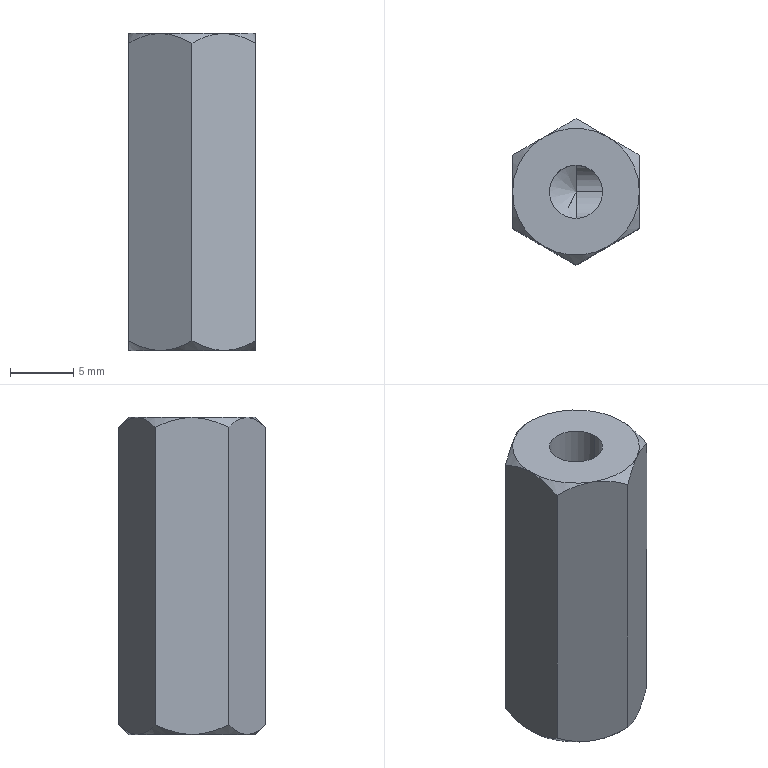Part | SolidWorks | features HoleWzd 3, RevCut 2, Extrusion 1, ICE 1 | 1 solid | 30 faces | box 10 x 11.547 x 25 mm | volume 1883 mm3 | cone 15 | plane 9 | cylinder 6 | commonest cylinder face diameters 4.2 x4 3.3 x2
STEP:
#1=CARTESIAN_POINT('',(1.65,0.,9.));
#2=VERTEX_POINT('',#1);
#3=CARTESIAN_POINT('',(-1.65,0.,9.));
#4=VERTEX_POINT('',#3);
#5=CARTESIAN_POINT('',(0.,0.,9.));
#6=DIRECTION('',(0.,0.,-1.));
#7=DIRECTION('',(-1.,0.,0.));
#8=AXIS2_PLACEMENT_3D('',#5,#6,#7);
#9=CIRCLE('',#8,1.65);
#10=EDGE_CURVE('',#2,#4,#9,.T.);
#11=ORIENTED_EDGE('',*,*,#10,.F.);
#12=CARTESIAN_POINT('',(1.65,0.,0.));
#13=VERTEX_POINT('',#12);
#14=CARTESIAN_POINT('',(1.65,0.,0.));
#15=DIRECTION('',(0.,0.,-1.));
#16=VECTOR('',#15,1000.);
#17=LINE('',#14,#16);
#18=EDGE_CURVE('',#2,#13,#17,.T.);
#19=ORIENTED_EDGE('',*,*,#18,.T.);
#20=CARTESIAN_POINT('',(-1.65,0.,0.));
#21=VERTEX_POINT('',#20);
#22=CARTESIAN_POINT('',(0.,0.,0.));
#23=DIRECTION('',(0.,0.,-1.));
#24=DIRECTION('',(-1.,0.,0.));
#25=AXIS2_PLACEMENT_3D('',#22,#23,#24);
#26=CIRCLE('',#25,1.65);
#27=EDGE_CURVE('',#13,#21,#26,.T.);
#28=ORIENTED_EDGE('',*,*,#27,.T.);
#29=CARTESIAN_POINT('',(-1.65,0.,0.));
#30=DIRECTION('',(0.,0.,-1.));
#31=VECTOR('',#30,1000.);
#32=LINE('',#29,#31);
#33=EDGE_CURVE('',#4,#21,#32,.T.);
#34=ORIENTED_EDGE('',*,*,#33,.F.);
#35=EDGE_LOOP('',(#11,#19,#28,#34));
#36=FACE_OUTER_BOUND('',#35,.T.);
#37=CARTESIAN_POINT('',(0.,0.,0.));
#38=DIRECTION('',(0.,0.,-1.));
#39=DIRECTION('',(-1.,0.,0.));
#40=AXIS2_PLACEMENT_3D('',#37,#38,#39);
#41=CYLINDRICAL_SURFACE('',#40,1.65);
#42=ADVANCED_FACE('',(#36),#41,.F.);
#43=CARTESIAN_POINT('',(0.,0.,9.991));
#44=VERTEX_POINT('',#43);
#45=CARTESIAN_POINT('',(-1.65,0.,9.));
#46=DIRECTION('',(-0.8572,0.,-0.515));
#47=VECTOR('',#46,1000.);
#48=LINE('',#45,#47);
#49=EDGE_CURVE('',#44,#4,#48,.T.);
#50=ORIENTED_EDGE('',*,*,#49,.F.);
#51=CARTESIAN_POINT('',(1.65,0.,9.));
#52=DIRECTION('',(0.8572,0.,-0.515));
#53=VECTOR('',#52,1000.);
#54=LINE('',#51,#53);
#55=EDGE_CURVE('',#44,#2,#54,.T.);
#56=ORIENTED_EDGE('',*,*,#55,.T.);
#57=ORIENTED_EDGE('',*,*,#10,.T.);
#58=EDGE_LOOP('',(#50,#56,#57));
#59=FACE_OUTER_BOUND('',#58,.T.);
#60=CARTESIAN_POINT('',(0.,0.,9.));
#61=DIRECTION('',(0.,0.,-1.));
#62=DIRECTION('',(-1.,0.,0.));
#63=AXIS2_PLACEMENT_3D('',#60,#61,#62);
#64=CONICAL_SURFACE('',#63,1.65,1.03);
#65=ADVANCED_FACE('',(#59),#64,.F.);
#66=CARTESIAN_POINT('',(5.,0.,12.9));
#67=VERTEX_POINT('',#66);
#68=CARTESIAN_POINT('',(5.,0.,17.1));
#69=VERTEX_POINT('',#68);
#70=CARTESIAN_POINT('',(5.,0.,15.));
#71=DIRECTION('',(-1.,0.,0.));
#72=DIRECTION('',(0.,0.,1.));
#73=AXIS2_PLACEMENT_3D('',#70,#71,#72);
#74=CIRCLE('',#73,2.1);
#75=EDGE_CURVE('',#67,#69,#74,.T.);
#76=ORIENTED_EDGE('',*,*,#75,.F.);
#77=CARTESIAN_POINT('',(0.,0.,12.9));
#78=VERTEX_POINT('',#77);
#79=CARTESIAN_POINT('',(0.,0.,12.9));
#80=DIRECTION('',(-1.,0.,0.));
#81=VECTOR('',#80,1000.);
#82=LINE('',#79,#81);
#83=EDGE_CURVE('',#67,#78,#82,.T.);
#84=ORIENTED_EDGE('',*,*,#83,.T.);
#85=CARTESIAN_POINT('',(0.,-2.1,15.));
#86=VERTEX_POINT('',#85);
#87=CARTESIAN_POINT('',(0.,0.,15.));
#88=DIRECTION('',(-1.,0.,0.));
#89=DIRECTION('',(0.,0.,1.));
#90=AXIS2_PLACEMENT_3D('',#87,#88,#89);
#91=CIRCLE('',#90,2.1);
#92=EDGE_CURVE('',#78,#86,#91,.T.);
#93=ORIENTED_EDGE('',*,*,#92,.T.);
#94=CARTESIAN_POINT('',(2.1,0.,17.1));
#95=VERTEX_POINT('',#94);
#96=CARTESIAN_POINT('',(2.1,0.,17.1));
#97=CARTESIAN_POINT('',(2.1,-1.23,17.1));
#98=CARTESIAN_POINT('',(1.23,-2.1,16.23));
#99=CARTESIAN_POINT('',(0.,-2.1,15.));
#100=(BOUNDED_CURVE()B_SPLINE_CURVE(3,(#96,#97,#98,#99),.UNSPECIFIED.,.F.,.T.)B_SPLINE_CURVE_WITH_KNOTS((4,4),(0.,1.571),.UNSPECIFIED.)CURVE()GEOMETRIC_REPRESENTATION_ITEM()RATIONAL_B_SPLINE_CURVE((1.,0.8047,0.8047,1.))REPRESENTATION_ITEM(''));
#101=EDGE_CURVE('',#95,#86,#100,.T.);
#102=ORIENTED_EDGE('',*,*,#101,.F.);
#103=CARTESIAN_POINT('',(0.,0.,17.1));
#104=DIRECTION('',(-1.,0.,0.));
#105=VECTOR('',#104,1000.);
#106=LINE('',#103,#105);
#107=EDGE_CURVE('',#69,#95,#106,.T.);
#108=ORIENTED_EDGE('',*,*,#107,.F.);
#109=EDGE_LOOP('',(#76,#84,#93,#102,#108));
#110=FACE_OUTER_BOUND('',#109,.T.);
#111=CARTESIAN_POINT('',(0.,0.,15.));
#112=DIRECTION('',(-1.,0.,0.));
#113=DIRECTION('',(0.,0.,1.));
#114=AXIS2_PLACEMENT_3D('',#111,#112,#113);
#115=CYLINDRICAL_SURFACE('',#114,2.1);
#116=ADVANCED_FACE('',(#110),#115,.F.);
#117=CARTESIAN_POINT('',(-2.1,0.,15.));
#118=VERTEX_POINT('',#117);
#119=CARTESIAN_POINT('',(0.,0.,15.));
#120=DIRECTION('',(0.,0.,1.));
#121=DIRECTION('',(1.,0.,0.));
#122=AXIS2_PLACEMENT_3D('',#119,#120,#121);
#123=CIRCLE('',#122,2.1);
#124=EDGE_CURVE('',#118,#86,#123,.T.);
#125=ORIENTED_EDGE('',*,*,#124,.F.);
#126=CARTESIAN_POINT('',(-2.1,0.,25.));
#127=VERTEX_POINT('',#126);
#128=CARTESIAN_POINT('',(-2.1,0.,25.));
#129=DIRECTION('',(0.,0.,1.));
#130=VECTOR('',#129,1000.);
#131=LINE('',#128,#130);
#132=EDGE_CURVE('',#118,#127,#131,.T.);
#133=ORIENTED_EDGE('',*,*,#132,.T.);
#134=CARTESIAN_POINT('',(2.1,0.,25.));
#135=VERTEX_POINT('',#134);
#136=CARTESIAN_POINT('',(0.,0.,25.));
#137=DIRECTION('',(0.,0.,1.));
#138=DIRECTION('',(1.,0.,0.));
#139=AXIS2_PLACEMENT_3D('',#136,#137,#138);
#140=CIRCLE('',#139,2.1);
#141=EDGE_CURVE('',#127,#135,#140,.T.);
#142=ORIENTED_EDGE('',*,*,#141,.T.);
#143=CARTESIAN_POINT('',(2.1,0.,25.));
#144=DIRECTION('',(0.,0.,1.));
#145=VECTOR('',#144,1000.);
#146=LINE('',#143,#145);
#147=EDGE_CURVE('',#95,#135,#146,.T.);
#148=ORIENTED_EDGE('',*,*,#147,.F.);
#149=ORIENTED_EDGE('',*,*,#101,.T.);
#150=EDGE_LOOP('',(#125,#133,#142,#148,#149));
#151=FACE_OUTER_BOUND('',#150,.T.);
#152=CARTESIAN_POINT('',(0.,0.,25.));
#153=DIRECTION('',(0.,0.,1.));
#154=DIRECTION('',(1.,0.,0.));
#155=AXIS2_PLACEMENT_3D('',#152,#153,#154);
#156=CYLINDRICAL_SURFACE('',#155,2.1);
#157=ADVANCED_FACE('',(#151),#156,.F.);
#158=CARTESIAN_POINT('',(5.,2.887,24.226));
#159=VERTEX_POINT('',#158);
#160=CARTESIAN_POINT('',(2.5,4.33,25.));
#161=VERTEX_POINT('',#160);
#162=CARTESIAN_POINT('',(5.,2.887,24.226));
#163=CARTESIAN_POINT('',(4.608,3.113,24.453));
#164=CARTESIAN_POINT('',(4.207,3.345,24.645));
#165=CARTESIAN_POINT('',(3.584,3.704,24.851));
#166=CARTESIAN_POINT('',(3.373,3.826,24.905));
#167=CARTESIAN_POINT('',(2.941,4.075,24.98));
#168=CARTESIAN_POINT('',(2.719,4.204,25.));
#169=CARTESIAN_POINT('',(2.5,4.33,25.));
#170=B_SPLINE_CURVE_WITH_KNOTS('',3,(#162,#163,#164,#165,#166,#167,#168,#169),.UNSPECIFIED.,.F.,.F.,(4,2,2,4),(0.000000254,0.001496,0.002245,0.002993),.UNSPECIFIED.);
#171=EDGE_CURVE('',#159,#161,#170,.T.);
#172=ORIENTED_EDGE('',*,*,#171,.F.);
#173=CARTESIAN_POINT('',(5.,2.887,0.7735));
#174=VERTEX_POINT('',#173);
#175=CARTESIAN_POINT('',(5.,2.887,25.));
#176=DIRECTION('',(0.,0.,-1.));
#177=VECTOR('',#176,1000.);
#178=LINE('',#175,#177);
#179=EDGE_CURVE('',#159,#174,#178,.T.);
#180=ORIENTED_EDGE('',*,*,#179,.T.);
#181=CARTESIAN_POINT('',(2.5,4.33,0.));
#182=VERTEX_POINT('',#181);
#183=CARTESIAN_POINT('',(2.5,4.33,0.));
#184=CARTESIAN_POINT('',(2.935,4.079,0.));
#185=CARTESIAN_POINT('',(3.362,3.832,0.07678));
#186=CARTESIAN_POINT('',(4.205,3.346,0.3535));
#187=CARTESIAN_POINT('',(4.608,3.113,0.5474));
#188=CARTESIAN_POINT('',(5.,2.887,0.7735));
#189=B_SPLINE_CURVE_WITH_KNOTS('',3,(#183,#184,#185,#186,#187,#188),.UNSPECIFIED.,.F.,.F.,(4,2,4),(0.002993,0.004478,0.005964),.UNSPECIFIED.);
#190=EDGE_CURVE('',#182,#174,#189,.T.);
#191=ORIENTED_EDGE('',*,*,#190,.F.);
#192=CARTESIAN_POINT('',(0.,5.774,0.7735));
#193=VERTEX_POINT('',#192);
#194=CARTESIAN_POINT('',(0.,5.774,0.7735));
#195=CARTESIAN_POINT('',(0.392,5.547,0.5472));
#196=CARTESIAN_POINT('',(0.7929,5.316,0.3548));
#197=CARTESIAN_POINT('',(1.416,4.956,0.1492));
#198=CARTESIAN_POINT('',(1.627,4.834,0.0946));
#199=CARTESIAN_POINT('',(2.059,4.585,0.01985));
#200=CARTESIAN_POINT('',(2.281,4.457,0.));
#201=CARTESIAN_POINT('',(2.5,4.33,0.));
#202=B_SPLINE_CURVE_WITH_KNOTS('',3,(#194,#195,#196,#197,#198,#199,#200,#201),.UNSPECIFIED.,.F.,.F.,(4,2,2,4),(0.000000254,0.001496,0.002245,0.002993),.UNSPECIFIED.);
#203=EDGE_CURVE('',#193,#182,#202,.T.);
#204=ORIENTED_EDGE('',*,*,#203,.F.);
#205=CARTESIAN_POINT('',(0.,5.774,24.226));
#206=VERTEX_POINT('',#205);
#207=CARTESIAN_POINT('',(0.,5.774,25.));
#208=DIRECTION('',(0.,0.,-1.));
#209=VECTOR('',#208,1000.);
#210=LINE('',#207,#209);
#211=EDGE_CURVE('',#206,#193,#210,.T.);
#212=ORIENTED_EDGE('',*,*,#211,.F.);
#213=CARTESIAN_POINT('',(2.5,4.33,25.));
#214=CARTESIAN_POINT('',(2.065,4.581,25.));
#215=CARTESIAN_POINT('',(1.638,4.828,24.923));
#216=CARTESIAN_POINT('',(0.7946,5.315,24.647));
#217=CARTESIAN_POINT('',(0.3916,5.547,24.453));
#218=CARTESIAN_POINT('',(0.,5.774,24.226));
#219=B_SPLINE_CURVE_WITH_KNOTS('',3,(#213,#214,#215,#216,#217,#218),.UNSPECIFIED.,.F.,.F.,(4,2,4),(0.002993,0.004478,0.005964),.UNSPECIFIED.);
#220=EDGE_CURVE('',#161,#206,#219,.T.);
#221=ORIENTED_EDGE('',*,*,#220,.F.);
#222=EDGE_LOOP('',(#172,#180,#191,#204,#212,#221));
#223=FACE_OUTER_BOUND('',#222,.T.);
#224=CARTESIAN_POINT('',(5.,2.887,25.));
#225=DIRECTION('',(-0.5,-0.866,0.));
#226=DIRECTION('',(0.866,-0.5,0.));
#227=AXIS2_PLACEMENT_3D('',#224,#225,#226);
#228=PLANE('',#227);
#229=ADVANCED_FACE('',(#223),#228,.F.);
#230=CARTESIAN_POINT('',(-2.5,4.33,25.));
#231=VERTEX_POINT('',#230);
#232=CARTESIAN_POINT('',(0.,5.774,24.226));
#233=CARTESIAN_POINT('',(-0.392,5.547,24.453));
#234=CARTESIAN_POINT('',(-0.7929,5.316,24.645));
#235=CARTESIAN_POINT('',(-1.416,4.956,24.851));
#236=CARTESIAN_POINT('',(-1.627,4.834,24.905));
#237=CARTESIAN_POINT('',(-2.059,4.585,24.98));
#238=CARTESIAN_POINT('',(-2.281,4.457,25.));
#239=CARTESIAN_POINT('',(-2.5,4.33,25.));
#240=B_SPLINE_CURVE_WITH_KNOTS('',3,(#232,#233,#234,#235,#236,#237,#238,#239),.UNSPECIFIED.,.F.,.F.,(4,2,2,4),(0.000000254,0.001496,0.002245,0.002993),.UNSPECIFIED.);
#241=EDGE_CURVE('',#206,#231,#240,.T.);
#242=ORIENTED_EDGE('',*,*,#241,.F.);
#243=ORIENTED_EDGE('',*,*,#211,.T.);
#244=CARTESIAN_POINT('',(-2.5,4.33,0.));
#245=VERTEX_POINT('',#244);
#246=CARTESIAN_POINT('',(-2.5,4.33,0.));
#247=CARTESIAN_POINT('',(-2.065,4.581,0.));
#248=CARTESIAN_POINT('',(-1.638,4.828,0.07678));
#249=CARTESIAN_POINT('',(-0.7946,5.315,0.3535));
#250=CARTESIAN_POINT('',(-0.3916,5.547,0.5474));
#251=CARTESIAN_POINT('',(0.,5.774,0.7735));
#252=B_SPLINE_CURVE_WITH_KNOTS('',3,(#246,#247,#248,#249,#250,#251),.UNSPECIFIED.,.F.,.F.,(4,2,4),(0.002993,0.004478,0.005964),.UNSPECIFIED.);
#253=EDGE_CURVE('',#245,#193,#252,.T.);
#254=ORIENTED_EDGE('',*,*,#253,.F.);
#255=CARTESIAN_POINT('',(-5.,2.887,0.7735));
#256=VERTEX_POINT('',#255);
#257=CARTESIAN_POINT('',(-5.,2.887,0.7735));
#258=CARTESIAN_POINT('',(-4.608,3.113,0.5472));
#259=CARTESIAN_POINT('',(-4.207,3.345,0.3548));
#260=CARTESIAN_POINT('',(-3.584,3.704,0.1492));
#261=CARTESIAN_POINT('',(-3.373,3.826,0.0946));
#262=CARTESIAN_POINT('',(-2.941,4.075,0.01985));
#263=CARTESIAN_POINT('',(-2.719,4.204,0.));
#264=CARTESIAN_POINT('',(-2.5,4.33,0.));
#265=B_SPLINE_CURVE_WITH_KNOTS('',3,(#257,#258,#259,#260,#261,#262,#263,#264),.UNSPECIFIED.,.F.,.F.,(4,2,2,4),(0.000000254,0.001496,0.002245,0.002993),.UNSPECIFIED.);
#266=EDGE_CURVE('',#256,#245,#265,.T.);
#267=ORIENTED_EDGE('',*,*,#266,.F.);
#268=CARTESIAN_POINT('',(-5.,2.887,24.226));
#269=VERTEX_POINT('',#268);
#270=CARTESIAN_POINT('',(-5.,2.887,25.));
#271=DIRECTION('',(0.,0.,-1.));
#272=VECTOR('',#271,1000.);
#273=LINE('',#270,#272);
#274=EDGE_CURVE('',#269,#256,#273,.T.);
#275=ORIENTED_EDGE('',*,*,#274,.F.);
#276=CARTESIAN_POINT('',(-2.5,4.33,25.));
#277=CARTESIAN_POINT('',(-2.935,4.079,25.));
#278=CARTESIAN_POINT('',(-3.362,3.832,24.923));
#279=CARTESIAN_POINT('',(-4.205,3.346,24.647));
#280=CARTESIAN_POINT('',(-4.608,3.113,24.453));
#281=CARTESIAN_POINT('',(-5.,2.887,24.226));
#282=B_SPLINE_CURVE_WITH_KNOTS('',3,(#276,#277,#278,#279,#280,#281),.UNSPECIFIED.,.F.,.F.,(4,2,4),(0.002993,0.004478,0.005964),.UNSPECIFIED.);
#283=EDGE_CURVE('',#231,#269,#282,.T.);
#284=ORIENTED_EDGE('',*,*,#283,.F.);
#285=EDGE_LOOP('',(#242,#243,#254,#267,#275,#284));
#286=FACE_OUTER_BOUND('',#285,.T.);
#287=CARTESIAN_POINT('',(0.,5.774,25.));
#288=DIRECTION('',(0.5,-0.866,0.));
#289=DIRECTION('',(0.866,0.5,0.));
#290=AXIS2_PLACEMENT_3D('',#287,#288,#289);
#291=PLANE('',#290);
#292=ADVANCED_FACE('',(#286),#291,.F.);
#293=CARTESIAN_POINT('',(-5.,0.,25.));
#294=VERTEX_POINT('',#293);
#295=CARTESIAN_POINT('',(-5.,2.887,24.226));
#296=CARTESIAN_POINT('',(-5.,2.663,24.338));
#297=CARTESIAN_POINT('',(-5.,2.435,24.443));
#298=CARTESIAN_POINT('',(-5.,1.967,24.631));
#299=CARTESIAN_POINT('',(-5.,1.726,24.715));
#300=CARTESIAN_POINT('',(-5.,1.001,24.922));
#301=CARTESIAN_POINT('',(-5.,0.5067,25.));
#302=CARTESIAN_POINT('',(-5.,0.,25.));
#303=B_SPLINE_CURVE_WITH_KNOTS('',3,(#295,#296,#297,#298,#299,#300,#301,#302),.UNSPECIFIED.,.F.,.F.,(4,2,2,4),(0.007249,0.008002,0.008755,0.01026),.UNSPECIFIED.);
#304=EDGE_CURVE('',#269,#294,#303,.T.);
#305=ORIENTED_EDGE('',*,*,#304,.F.);
#306=ORIENTED_EDGE('',*,*,#274,.T.);
#307=CARTESIAN_POINT('',(-5.,0.,0.));
#308=VERTEX_POINT('',#307);
#309=CARTESIAN_POINT('',(-5.,0.,0.));
#310=CARTESIAN_POINT('',(-5.,0.2527,0.));
#311=CARTESIAN_POINT('',(-5.,0.5069,0.01965));
#312=CARTESIAN_POINT('',(-5.,1.003,0.09364));
#313=CARTESIAN_POINT('',(-5.,1.246,0.1479));
#314=CARTESIAN_POINT('',(-5.,1.968,0.3536));
#315=CARTESIAN_POINT('',(-5.,2.439,0.5496));
#316=CARTESIAN_POINT('',(-5.,2.887,0.7735));
#317=B_SPLINE_CURVE_WITH_KNOTS('',3,(#309,#310,#311,#312,#313,#314,#315,#316),.UNSPECIFIED.,.F.,.F.,(4,2,2,4),(0.01026,0.01101,0.01176,0.01326),.UNSPECIFIED.);
#318=EDGE_CURVE('',#308,#256,#317,.T.);
#319=ORIENTED_EDGE('',*,*,#318,.F.);
#320=CARTESIAN_POINT('',(-5.,-2.887,0.7735));
#321=VERTEX_POINT('',#320);
#322=CARTESIAN_POINT('',(-5.,-2.887,0.7735));
#323=CARTESIAN_POINT('',(-5.,-2.663,0.6617));
#324=CARTESIAN_POINT('',(-5.,-2.435,0.5573));
#325=CARTESIAN_POINT('',(-5.,-1.967,0.3688));
#326=CARTESIAN_POINT('',(-5.,-1.726,0.2846));
#327=CARTESIAN_POINT('',(-5.,-1.001,0.07798));
#328=CARTESIAN_POINT('',(-5.,-0.5067,0.));
#329=CARTESIAN_POINT('',(-5.,0.,0.));
#330=B_SPLINE_CURVE_WITH_KNOTS('',3,(#322,#323,#324,#325,#326,#327,#328,#329),.UNSPECIFIED.,.F.,.F.,(4,2,2,4),(0.007249,0.008002,0.008755,0.01026),.UNSPECIFIED.);
#331=EDGE_CURVE('',#321,#308,#330,.T.);
#332=ORIENTED_EDGE('',*,*,#331,.F.);
#333=CARTESIAN_POINT('',(-5.,-2.887,24.226));
#334=VERTEX_POINT('',#333);
#335=CARTESIAN_POINT('',(-5.,-2.887,25.));
#336=DIRECTION('',(0.,0.,-1.));
#337=VECTOR('',#336,1000.);
#338=LINE('',#335,#337);
#339=EDGE_CURVE('',#334,#321,#338,.T.);
#340=ORIENTED_EDGE('',*,*,#339,.F.);
#341=CARTESIAN_POINT('',(-5.,0.,25.));
#342=CARTESIAN_POINT('',(-5.,-0.2527,25.));
#343=CARTESIAN_POINT('',(-5.,-0.5069,24.98));
#344=CARTESIAN_POINT('',(-5.,-1.003,24.906));
#345=CARTESIAN_POINT('',(-5.,-1.246,24.852));
#346=CARTESIAN_POINT('',(-5.,-1.968,24.646));
#347=CARTESIAN_POINT('',(-5.,-2.439,24.45));
#348=CARTESIAN_POINT('',(-5.,-2.887,24.226));
#349=B_SPLINE_CURVE_WITH_KNOTS('',3,(#341,#342,#343,#344,#345,#346,#347,#348),.UNSPECIFIED.,.F.,.F.,(4,2,2,4),(0.01026,0.01101,0.01176,0.01326),.UNSPECIFIED.);
#350=EDGE_CURVE('',#294,#334,#349,.T.);
#351=ORIENTED_EDGE('',*,*,#350,.F.);
#352=EDGE_LOOP('',(#305,#306,#319,#332,#340,#351));
#353=FACE_OUTER_BOUND('',#352,.T.);
#354=CARTESIAN_POINT('',(-5.,2.887,25.));
#355=DIRECTION('',(1.,0.,0.));
#356=DIRECTION('',(0.,1.,0.));
#357=AXIS2_PLACEMENT_3D('',#354,#355,#356);
#358=PLANE('',#357);
#359=ADVANCED_FACE('',(#353),#358,.F.);
#360=CARTESIAN_POINT('',(-2.5,-4.33,25.));
#361=VERTEX_POINT('',#360);
#362=CARTESIAN_POINT('',(-5.,-2.887,24.226));
#363=CARTESIAN_POINT('',(-4.608,-3.113,24.453));
#364=CARTESIAN_POINT('',(-4.207,-3.345,24.645));
#365=CARTESIAN_POINT('',(-3.584,-3.704,24.851));
#366=CARTESIAN_POINT('',(-3.373,-3.826,24.905));
#367=CARTESIAN_POINT('',(-2.941,-4.075,24.98));
#368=CARTESIAN_POINT('',(-2.719,-4.204,25.));
#369=CARTESIAN_POINT('',(-2.5,-4.33,25.));
#370=B_SPLINE_CURVE_WITH_KNOTS('',3,(#362,#363,#364,#365,#366,#367,#368,#369),.UNSPECIFIED.,.F.,.F.,(4,2,2,4),(0.000000254,0.001496,0.002245,0.002993),.UNSPECIFIED.);
#371=EDGE_CURVE('',#334,#361,#370,.T.);
#372=ORIENTED_EDGE('',*,*,#371,.F.);
#373=ORIENTED_EDGE('',*,*,#339,.T.);
#374=CARTESIAN_POINT('',(-2.5,-4.33,0.));
#375=VERTEX_POINT('',#374);
#376=CARTESIAN_POINT('',(-2.5,-4.33,0.));
#377=CARTESIAN_POINT('',(-2.935,-4.079,0.));
#378=CARTESIAN_POINT('',(-3.362,-3.832,0.07678));
#379=CARTESIAN_POINT('',(-4.205,-3.346,0.3535));
#380=CARTESIAN_POINT('',(-4.608,-3.113,0.5474));
#381=CARTESIAN_POINT('',(-5.,-2.887,0.7735));
#382=B_SPLINE_CURVE_WITH_KNOTS('',3,(#376,#377,#378,#379,#380,#381),.UNSPECIFIED.,.F.,.F.,(4,2,4),(0.002993,0.004478,0.005964),.UNSPECIFIED.);
#383=EDGE_CURVE('',#375,#321,#382,.T.);
#384=ORIENTED_EDGE('',*,*,#383,.F.);
#385=CARTESIAN_POINT('',(0.,-5.774,0.7735));
#386=VERTEX_POINT('',#385);
#387=CARTESIAN_POINT('',(0.,-5.774,0.7735));
#388=CARTESIAN_POINT('',(-0.392,-5.547,0.5472));
#389=CARTESIAN_POINT('',(-0.7929,-5.316,0.3548));
#390=CARTESIAN_POINT('',(-1.416,-4.956,0.1492));
#391=CARTESIAN_POINT('',(-1.627,-4.834,0.0946));
#392=CARTESIAN_POINT('',(-2.059,-4.585,0.01985));
#393=CARTESIAN_POINT('',(-2.281,-4.457,0.));
#394=CARTESIAN_POINT('',(-2.5,-4.33,0.));
#395=B_SPLINE_CURVE_WITH_KNOTS('',3,(#387,#388,#389,#390,#391,#392,#393,#394),.UNSPECIFIED.,.F.,.F.,(4,2,2,4),(0.000000254,0.001496,0.002245,0.002993),.UNSPECIFIED.);
#396=EDGE_CURVE('',#386,#375,#395,.T.);
#397=ORIENTED_EDGE('',*,*,#396,.F.);
#398=CARTESIAN_POINT('',(0.,-5.774,24.226));
#399=VERTEX_POINT('',#398);
#400=CARTESIAN_POINT('',(0.,-5.774,25.));
#401=DIRECTION('',(0.,0.,-1.));
#402=VECTOR('',#401,1000.);
#403=LINE('',#400,#402);
#404=EDGE_CURVE('',#399,#386,#403,.T.);
#405=ORIENTED_EDGE('',*,*,#404,.F.);
#406=CARTESIAN_POINT('',(-2.5,-4.33,25.));
#407=CARTESIAN_POINT('',(-2.065,-4.581,25.));
#408=CARTESIAN_POINT('',(-1.638,-4.828,24.923));
#409=CARTESIAN_POINT('',(-0.7946,-5.315,24.647));
#410=CARTESIAN_POINT('',(-0.3916,-5.547,24.453));
#411=CARTESIAN_POINT('',(0.,-5.774,24.226));
#412=B_SPLINE_CURVE_WITH_KNOTS('',3,(#406,#407,#408,#409,#410,#411),.UNSPECIFIED.,.F.,.F.,(4,2,4),(0.002993,0.004478,0.005964),.UNSPECIFIED.);
#413=EDGE_CURVE('',#361,#399,#412,.T.);
#414=ORIENTED_EDGE('',*,*,#413,.F.);
#415=EDGE_LOOP('',(#372,#373,#384,#397,#405,#414));
#416=FACE_OUTER_BOUND('',#415,.T.);
#417=CARTESIAN_POINT('',(-5.,-2.887,25.));
#418=DIRECTION('',(0.5,0.866,0.));
#419=DIRECTION('',(-0.866,0.5,0.));
#420=AXIS2_PLACEMENT_3D('',#417,#418,#419);
#421=PLANE('',#420);
#422=ADVANCED_FACE('',(#416),#421,.F.);
#423=CARTESIAN_POINT('',(2.5,-4.33,25.));
#424=VERTEX_POINT('',#423);
#425=CARTESIAN_POINT('',(0.,-5.774,24.226));
#426=CARTESIAN_POINT('',(0.392,-5.547,24.453));
#427=CARTESIAN_POINT('',(0.7929,-5.316,24.645));
#428=CARTESIAN_POINT('',(1.416,-4.956,24.851));
#429=CARTESIAN_POINT('',(1.627,-4.834,24.905));
#430=CARTESIAN_POINT('',(2.059,-4.585,24.98));
#431=CARTESIAN_POINT('',(2.281,-4.457,25.));
#432=CARTESIAN_POINT('',(2.5,-4.33,25.));
#433=B_SPLINE_CURVE_WITH_KNOTS('',3,(#425,#426,#427,#428,#429,#430,#431,#432),.UNSPECIFIED.,.F.,.F.,(4,2,2,4),(0.000000254,0.001496,0.002245,0.002993),.UNSPECIFIED.);
#434=EDGE_CURVE('',#399,#424,#433,.T.);
#435=ORIENTED_EDGE('',*,*,#434,.F.);
#436=ORIENTED_EDGE('',*,*,#404,.T.);
#437=CARTESIAN_POINT('',(2.5,-4.33,0.));
#438=VERTEX_POINT('',#437);
#439=CARTESIAN_POINT('',(2.5,-4.33,0.));
#440=CARTESIAN_POINT('',(2.065,-4.581,0.));
#441=CARTESIAN_POINT('',(1.638,-4.828,0.07678));
#442=CARTESIAN_POINT('',(0.7946,-5.315,0.3535));
#443=CARTESIAN_POINT('',(0.3916,-5.547,0.5474));
#444=CARTESIAN_POINT('',(0.,-5.774,0.7735));
#445=B_SPLINE_CURVE_WITH_KNOTS('',3,(#439,#440,#441,#442,#443,#444),.UNSPECIFIED.,.F.,.F.,(4,2,4),(0.002993,0.004478,0.005964),.UNSPECIFIED.);
#446=EDGE_CURVE('',#438,#386,#445,.T.);
#447=ORIENTED_EDGE('',*,*,#446,.F.);
#448=CARTESIAN_POINT('',(5.,-2.887,0.7735));
#449=VERTEX_POINT('',#448);
#450=CARTESIAN_POINT('',(5.,-2.887,0.7735));
#451=CARTESIAN_POINT('',(4.608,-3.113,0.5472));
#452=CARTESIAN_POINT('',(4.207,-3.345,0.3548));
#453=CARTESIAN_POINT('',(3.584,-3.704,0.1492));
#454=CARTESIAN_POINT('',(3.373,-3.826,0.0946));
#455=CARTESIAN_POINT('',(2.941,-4.075,0.01985));
#456=CARTESIAN_POINT('',(2.719,-4.204,0.));
#457=CARTESIAN_POINT('',(2.5,-4.33,0.));
#458=B_SPLINE_CURVE_WITH_KNOTS('',3,(#450,#451,#452,#453,#454,#455,#456,#457),.UNSPECIFIED.,.F.,.F.,(4,2,2,4),(0.000000254,0.001496,0.002245,0.002993),.UNSPECIFIED.);
#459=EDGE_CURVE('',#449,#438,#458,.T.);
#460=ORIENTED_EDGE('',*,*,#459,.F.);
#461=CARTESIAN_POINT('',(5.,-2.887,24.226));
#462=VERTEX_POINT('',#461);
#463=CARTESIAN_POINT('',(5.,-2.887,25.));
#464=DIRECTION('',(0.,0.,-1.));
#465=VECTOR('',#464,1000.);
#466=LINE('',#463,#465);
#467=EDGE_CURVE('',#462,#449,#466,.T.);
#468=ORIENTED_EDGE('',*,*,#467,.F.);
#469=CARTESIAN_POINT('',(2.5,-4.33,25.));
#470=CARTESIAN_POINT('',(2.935,-4.079,25.));
#471=CARTESIAN_POINT('',(3.362,-3.832,24.923));
#472=CARTESIAN_POINT('',(4.205,-3.346,24.647));
#473=CARTESIAN_POINT('',(4.608,-3.113,24.453));
#474=CARTESIAN_POINT('',(5.,-2.887,24.226));
#475=B_SPLINE_CURVE_WITH_KNOTS('',3,(#469,#470,#471,#472,#473,#474),.UNSPECIFIED.,.F.,.F.,(4,2,4),(0.002993,0.004478,0.005964),.UNSPECIFIED.);
#476=EDGE_CURVE('',#424,#462,#475,.T.);
#477=ORIENTED_EDGE('',*,*,#476,.F.);
#478=EDGE_LOOP('',(#435,#436,#447,#460,#468,#477));
#479=FACE_OUTER_BOUND('',#478,.T.);
#480=CARTESIAN_POINT('',(0.,-5.774,25.));
#481=DIRECTION('',(-0.5,0.866,0.));
#482=DIRECTION('',(-0.866,-0.5,0.));
#483=AXIS2_PLACEMENT_3D('',#480,#481,#482);
#484=PLANE('',#483);
#485=ADVANCED_FACE('',(#479),#484,.F.);
#486=CARTESIAN_POINT('',(5.,0.,15.));
#487=DIRECTION('',(-1.,0.,0.));
#488=DIRECTION('',(0.,0.,1.));
#489=AXIS2_PLACEMENT_3D('',#486,#487,#488);
#490=CIRCLE('',#489,2.1);
#491=EDGE_CURVE('',#69,#67,#490,.T.);
#492=ORIENTED_EDGE('',*,*,#491,.T.);
#493=ORIENTED_EDGE('',*,*,#75,.T.);
#494=EDGE_LOOP('',(#492,#493));
#495=FACE_BOUND('',#494,.T.);
#496=CARTESIAN_POINT('',(5.,0.,25.));
#497=VERTEX_POINT('',#496);
#498=CARTESIAN_POINT('',(5.,-2.887,24.226));
#499=CARTESIAN_POINT('',(5.,-2.663,24.338));
#500=CARTESIAN_POINT('',(5.,-2.435,24.443));
#501=CARTESIAN_POINT('',(5.,-1.967,24.631));
#502=CARTESIAN_POINT('',(5.,-1.726,24.715));
#503=CARTESIAN_POINT('',(5.,-1.001,24.922));
#504=CARTESIAN_POINT('',(5.,-0.5067,25.));
#505=CARTESIAN_POINT('',(5.,0.,25.));
#506=B_SPLINE_CURVE_WITH_KNOTS('',3,(#498,#499,#500,#501,#502,#503,#504,#505),.UNSPECIFIED.,.F.,.F.,(4,2,2,4),(0.007249,0.008002,0.008755,0.01026),.UNSPECIFIED.);
#507=EDGE_CURVE('',#462,#497,#506,.T.);
#508=ORIENTED_EDGE('',*,*,#507,.F.);
#509=ORIENTED_EDGE('',*,*,#467,.T.);
#510=CARTESIAN_POINT('',(5.,0.,0.));
#511=VERTEX_POINT('',#510);
#512=CARTESIAN_POINT('',(5.,0.,0.));
#513=CARTESIAN_POINT('',(5.,-0.2527,0.));
#514=CARTESIAN_POINT('',(5.,-0.5069,0.01965));
#515=CARTESIAN_POINT('',(5.,-1.003,0.09364));
#516=CARTESIAN_POINT('',(5.,-1.246,0.1479));
#517=CARTESIAN_POINT('',(5.,-1.968,0.3536));
#518=CARTESIAN_POINT('',(5.,-2.439,0.5496));
#519=CARTESIAN_POINT('',(5.,-2.887,0.7735));
#520=B_SPLINE_CURVE_WITH_KNOTS('',3,(#512,#513,#514,#515,#516,#517,#518,#519),.UNSPECIFIED.,.F.,.F.,(4,2,2,4),(0.01026,0.01101,0.01176,0.01326),.UNSPECIFIED.);
#521=EDGE_CURVE('',#511,#449,#520,.T.);
#522=ORIENTED_EDGE('',*,*,#521,.F.);
#523=CARTESIAN_POINT('',(5.,2.887,0.7735));
#524=CARTESIAN_POINT('',(5.,2.663,0.6617));
#525=CARTESIAN_POINT('',(5.,2.435,0.5573));
#526=CARTESIAN_POINT('',(5.,1.967,0.3688));
#527=CARTESIAN_POINT('',(5.,1.726,0.2846));
#528=CARTESIAN_POINT('',(5.,1.001,0.07798));
#529=CARTESIAN_POINT('',(5.,0.5067,0.));
#530=CARTESIAN_POINT('',(5.,0.,0.));
#531=B_SPLINE_CURVE_WITH_KNOTS('',3,(#523,#524,#525,#526,#527,#528,#529,#530),.UNSPECIFIED.,.F.,.F.,(4,2,2,4),(0.007249,0.008002,0.008755,0.01026),.UNSPECIFIED.);
#532=EDGE_CURVE('',#174,#511,#531,.T.);
#533=ORIENTED_EDGE('',*,*,#532,.F.);
#534=ORIENTED_EDGE('',*,*,#179,.F.);
#535=CARTESIAN_POINT('',(5.,0.,25.));
#536=CARTESIAN_POINT('',(5.,0.2527,25.));
#537=CARTESIAN_POINT('',(5.,0.5069,24.98));
#538=CARTESIAN_POINT('',(5.,1.003,24.906));
#539=CARTESIAN_POINT('',(5.,1.246,24.852));
#540=CARTESIAN_POINT('',(5.,1.968,24.646));
#541=CARTESIAN_POINT('',(5.,2.439,24.45));
#542=CARTESIAN_POINT('',(5.,2.887,24.226));
#543=B_SPLINE_CURVE_WITH_KNOTS('',3,(#535,#536,#537,#538,#539,#540,#541,#542),.UNSPECIFIED.,.F.,.F.,(4,2,2,4),(0.01026,0.01101,0.01176,0.01326),.UNSPECIFIED.);
#544=EDGE_CURVE('',#497,#159,#543,.T.);
#545=ORIENTED_EDGE('',*,*,#544,.F.);
#546=EDGE_LOOP('',(#508,#509,#522,#533,#534,#545));
#547=FACE_OUTER_BOUND('',#546,.T.);
#548=CARTESIAN_POINT('',(5.,-2.887,25.));
#549=DIRECTION('',(-1.,0.,0.));
#550=DIRECTION('',(0.,-1.,0.));
#551=AXIS2_PLACEMENT_3D('',#548,#549,#550);
#552=PLANE('',#551);
#553=ADVANCED_FACE('',(#495,#547),#552,.F.);
#554=CARTESIAN_POINT('',(0.,0.,25.));
#555=DIRECTION('',(0.,0.,1.));
#556=DIRECTION('',(1.,0.,0.));
#557=AXIS2_PLACEMENT_3D('',#554,#555,#556);
#558=CIRCLE('',#557,2.1);
#559=EDGE_CURVE('',#135,#127,#558,.T.);
#560=ORIENTED_EDGE('',*,*,#559,.F.);
#561=ORIENTED_EDGE('',*,*,#141,.F.);
#562=EDGE_LOOP('',(#560,#561));
#563=FACE_BOUND('',#562,.T.);
#564=CARTESIAN_POINT('',(0.,0.,25.));
#565=DIRECTION('',(0.,0.,1.));
#566=DIRECTION('',(1.,0.,0.));
#567=AXIS2_PLACEMENT_3D('',#564,#565,#566);
#568=CIRCLE('',#567,5.);
#569=EDGE_CURVE('',#424,#497,#568,.T.);
#570=ORIENTED_EDGE('',*,*,#569,.T.);
#571=CARTESIAN_POINT('',(0.,0.,25.));
#572=DIRECTION('',(0.,0.,1.));
#573=DIRECTION('',(1.,0.,0.));
#574=AXIS2_PLACEMENT_3D('',#571,#572,#573);
#575=CIRCLE('',#574,5.);
#576=EDGE_CURVE('',#497,#161,#575,.T.);
#577=ORIENTED_EDGE('',*,*,#576,.T.);
#578=CARTESIAN_POINT('',(0.,0.,25.));
#579=DIRECTION('',(0.,0.,1.));
#580=DIRECTION('',(1.,0.,0.));
#581=AXIS2_PLACEMENT_3D('',#578,#579,#580);
#582=CIRCLE('',#581,5.);
#583=EDGE_CURVE('',#161,#231,#582,.T.);
#584=ORIENTED_EDGE('',*,*,#583,.T.);
#585=CARTESIAN_POINT('',(0.,0.,25.));
#586=DIRECTION('',(0.,0.,1.));
#587=DIRECTION('',(1.,0.,0.));
#588=AXIS2_PLACEMENT_3D('',#585,#586,#587);
#589=CIRCLE('',#588,5.);
#590=EDGE_CURVE('',#231,#294,#589,.T.);
#591=ORIENTED_EDGE('',*,*,#590,.T.);
#592=CARTESIAN_POINT('',(0.,0.,25.));
#593=DIRECTION('',(0.,0.,1.));
#594=DIRECTION('',(1.,0.,0.));
#595=AXIS2_PLACEMENT_3D('',#592,#593,#594);
#596=CIRCLE('',#595,5.);
#597=EDGE_CURVE('',#294,#361,#596,.T.);
#598=ORIENTED_EDGE('',*,*,#597,.T.);
#599=CARTESIAN_POINT('',(0.,0.,25.));
#600=DIRECTION('',(0.,0.,1.));
#601=DIRECTION('',(1.,0.,0.));
#602=AXIS2_PLACEMENT_3D('',#599,#600,#601);
#603=CIRCLE('',#602,5.);
#604=EDGE_CURVE('',#361,#424,#603,.T.);
#605=ORIENTED_EDGE('',*,*,#604,.T.);
#606=EDGE_LOOP('',(#570,#577,#584,#591,#598,#605));
#607=FACE_OUTER_BOUND('',#606,.T.);
#608=CARTESIAN_POINT('',(0.,0.,25.));
#609=DIRECTION('',(0.,0.,1.));
#610=DIRECTION('',(1.,0.,0.));
#611=AXIS2_PLACEMENT_3D('',#608,#609,#610);
#612=PLANE('',#611);
#613=ADVANCED_FACE('',(#563,#607),#612,.T.);
#614=CARTESIAN_POINT('',(0.,2.1,15.));
#615=VERTEX_POINT('',#614);
#616=CARTESIAN_POINT('',(0.,0.,15.));
#617=DIRECTION('',(0.,0.,1.));
#618=DIRECTION('',(1.,0.,0.));
#619=AXIS2_PLACEMENT_3D('',#616,#617,#618);
#620=CIRCLE('',#619,2.1);
#621=EDGE_CURVE('',#615,#118,#620,.T.);
#622=ORIENTED_EDGE('',*,*,#621,.T.);
#623=ORIENTED_EDGE('',*,*,#124,.T.);
#624=CARTESIAN_POINT('',(0.,0.,13.738));
#625=VERTEX_POINT('',#624);
#626=CARTESIAN_POINT('',(0.,0.,13.738));
#627=DIRECTION('',(0.,0.8572,-0.515));
#628=VECTOR('',#627,1000.);
#629=LINE('',#626,#628);
#630=EDGE_CURVE('',#86,#625,#629,.T.);
#631=ORIENTED_EDGE('',*,*,#630,.T.);
#632=CARTESIAN_POINT('',(0.,0.,13.738));
#633=DIRECTION('',(0.,0.8572,0.515));
#634=VECTOR('',#633,1000.);
#635=LINE('',#632,#634);
#636=EDGE_CURVE('',#625,#615,#635,.T.);
#637=ORIENTED_EDGE('',*,*,#636,.T.);
#638=EDGE_LOOP('',(#622,#623,#631,#637));
#639=FACE_OUTER_BOUND('',#638,.T.);
#640=CARTESIAN_POINT('',(0.,0.,15.));
#641=DIRECTION('',(0.,0.,1.));
#642=DIRECTION('',(1.,0.,0.));
#643=AXIS2_PLACEMENT_3D('',#640,#641,#642);
#644=CONICAL_SURFACE('',#643,2.1,1.03);
#645=ADVANCED_FACE('',(#639),#644,.F.);
#646=ORIENTED_EDGE('',*,*,#132,.F.);
#647=ORIENTED_EDGE('',*,*,#621,.F.);
#648=CARTESIAN_POINT('',(0.,2.1,15.));
#649=CARTESIAN_POINT('',(1.23,2.1,16.23));
#650=CARTESIAN_POINT('',(2.1,1.23,17.1));
#651=CARTESIAN_POINT('',(2.1,0.,17.1));
#652=(BOUNDED_CURVE()B_SPLINE_CURVE(3,(#648,#649,#650,#651),.UNSPECIFIED.,.F.,.T.)B_SPLINE_CURVE_WITH_KNOTS((4,4),(4.712,6.283),.UNSPECIFIED.)CURVE()GEOMETRIC_REPRESENTATION_ITEM()RATIONAL_B_SPLINE_CURVE((1.,0.8047,0.8047,1.))REPRESENTATION_ITEM(''));
#653=EDGE_CURVE('',#615,#95,#652,.T.);
#654=ORIENTED_EDGE('',*,*,#653,.T.);
#655=ORIENTED_EDGE('',*,*,#147,.T.);
#656=ORIENTED_EDGE('',*,*,#559,.T.);
#657=EDGE_LOOP('',(#646,#647,#654,#655,#656));
#658=FACE_OUTER_BOUND('',#657,.T.);
#659=CARTESIAN_POINT('',(0.,0.,25.));
#660=DIRECTION('',(0.,0.,1.));
#661=DIRECTION('',(1.,0.,0.));
#662=AXIS2_PLACEMENT_3D('',#659,#660,#661);
#663=CYLINDRICAL_SURFACE('',#662,2.1);
#664=ADVANCED_FACE('',(#658),#663,.F.);
#665=CARTESIAN_POINT('',(0.,0.,15.));
#666=DIRECTION('',(-1.,0.,0.));
#667=DIRECTION('',(0.,0.,1.));
#668=AXIS2_PLACEMENT_3D('',#665,#666,#667);
#669=CIRCLE('',#668,2.1);
#670=EDGE_CURVE('',#615,#78,#669,.T.);
#671=ORIENTED_EDGE('',*,*,#670,.F.);
#672=ORIENTED_EDGE('',*,*,#636,.F.);
#673=ORIENTED_EDGE('',*,*,#630,.F.);
#674=ORIENTED_EDGE('',*,*,#92,.F.);
#675=EDGE_LOOP('',(#671,#672,#673,#674));
#676=FACE_OUTER_BOUND('',#675,.T.);
#677=CARTESIAN_POINT('',(0.,2.1,15.));
#678=DIRECTION('',(-1.,0.,0.));
#679=DIRECTION('',(0.,0.,1.));
#680=AXIS2_PLACEMENT_3D('',#677,#678,#679);
#681=PLANE('',#680);
#682=ADVANCED_FACE('',(#676),#681,.F.);
#683=ORIENTED_EDGE('',*,*,#83,.F.);
#684=ORIENTED_EDGE('',*,*,#491,.F.);
#685=ORIENTED_EDGE('',*,*,#107,.T.);
#686=ORIENTED_EDGE('',*,*,#653,.F.);
#687=ORIENTED_EDGE('',*,*,#670,.T.);
#688=EDGE_LOOP('',(#683,#684,#685,#686,#687));
#689=FACE_OUTER_BOUND('',#688,.T.);
#690=CARTESIAN_POINT('',(0.,0.,15.));
#691=DIRECTION('',(-1.,0.,0.));
#692=DIRECTION('',(0.,0.,1.));
#693=AXIS2_PLACEMENT_3D('',#690,#691,#692);
#694=CYLINDRICAL_SURFACE('',#693,2.1);
#695=ADVANCED_FACE('',(#689),#694,.F.);
#696=ORIENTED_EDGE('',*,*,#459,.T.);
#697=CARTESIAN_POINT('',(0.,0.,0.));
#698=DIRECTION('',(0.,0.,1.));
#699=DIRECTION('',(1.,0.,0.));
#700=AXIS2_PLACEMENT_3D('',#697,#698,#699);
#701=CIRCLE('',#700,5.);
#702=EDGE_CURVE('',#438,#511,#701,.T.);
#703=ORIENTED_EDGE('',*,*,#702,.T.);
#704=ORIENTED_EDGE('',*,*,#521,.T.);
#705=EDGE_LOOP('',(#696,#703,#704));
#706=FACE_OUTER_BOUND('',#705,.T.);
#707=CARTESIAN_POINT('',(0.,0.,0.7735));
#708=DIRECTION('',(0.,0.,1.));
#709=DIRECTION('',(1.,0.,0.));
#710=AXIS2_PLACEMENT_3D('',#707,#708,#709);
#711=CONICAL_SURFACE('',#710,5.774,0.7854);
#712=ADVANCED_FACE('',(#706),#711,.T.);
#713=ORIENTED_EDGE('',*,*,#396,.T.);
#714=CARTESIAN_POINT('',(0.,0.,0.));
#715=DIRECTION('',(0.,0.,1.));
#716=DIRECTION('',(1.,0.,0.));
#717=AXIS2_PLACEMENT_3D('',#714,#715,#716);
#718=CIRCLE('',#717,5.);
#719=EDGE_CURVE('',#375,#438,#718,.T.);
#720=ORIENTED_EDGE('',*,*,#719,.T.);
#721=ORIENTED_EDGE('',*,*,#446,.T.);
#722=EDGE_LOOP('',(#713,#720,#721));
#723=FACE_OUTER_BOUND('',#722,.T.);
#724=CARTESIAN_POINT('',(0.,0.,0.7735));
#725=DIRECTION('',(0.,0.,1.));
#726=DIRECTION('',(1.,0.,0.));
#727=AXIS2_PLACEMENT_3D('',#724,#725,#726);
#728=CONICAL_SURFACE('',#727,5.774,0.7854);
#729=ADVANCED_FACE('',(#723),#728,.T.);
#730=ORIENTED_EDGE('',*,*,#331,.T.);
#731=CARTESIAN_POINT('',(0.,0.,0.));
#732=DIRECTION('',(0.,0.,1.));
#733=DIRECTION('',(1.,0.,0.));
#734=AXIS2_PLACEMENT_3D('',#731,#732,#733);
#735=CIRCLE('',#734,5.);
#736=EDGE_CURVE('',#308,#375,#735,.T.);
#737=ORIENTED_EDGE('',*,*,#736,.T.);
#738=ORIENTED_EDGE('',*,*,#383,.T.);
#739=EDGE_LOOP('',(#730,#737,#738));
#740=FACE_OUTER_BOUND('',#739,.T.);
#741=CARTESIAN_POINT('',(0.,0.,0.7735));
#742=DIRECTION('',(0.,0.,1.));
#743=DIRECTION('',(1.,0.,0.));
#744=AXIS2_PLACEMENT_3D('',#741,#742,#743);
#745=CONICAL_SURFACE('',#744,5.774,0.7854);
#746=ADVANCED_FACE('',(#740),#745,.T.);
#747=ORIENTED_EDGE('',*,*,#318,.T.);
#748=ORIENTED_EDGE('',*,*,#266,.T.);
#749=CARTESIAN_POINT('',(0.,0.,0.));
#750=DIRECTION('',(0.,0.,1.));
#751=DIRECTION('',(1.,0.,0.));
#752=AXIS2_PLACEMENT_3D('',#749,#750,#751);
#753=CIRCLE('',#752,5.);
#754=EDGE_CURVE('',#245,#308,#753,.T.);
#755=ORIENTED_EDGE('',*,*,#754,.T.);
#756=EDGE_LOOP('',(#747,#748,#755));
#757=FACE_OUTER_BOUND('',#756,.T.);
#758=CARTESIAN_POINT('',(0.,0.,0.7735));
#759=DIRECTION('',(0.,0.,1.));
#760=DIRECTION('',(1.,0.,0.));
#761=AXIS2_PLACEMENT_3D('',#758,#759,#760);
#762=CONICAL_SURFACE('',#761,5.774,0.7854);
#763=ADVANCED_FACE('',(#757),#762,.T.);
#764=ORIENTED_EDGE('',*,*,#253,.T.);
#765=ORIENTED_EDGE('',*,*,#203,.T.);
#766=CARTESIAN_POINT('',(0.,0.,0.));
#767=DIRECTION('',(0.,0.,1.));
#768=DIRECTION('',(1.,0.,0.));
#769=AXIS2_PLACEMENT_3D('',#766,#767,#768);
#770=CIRCLE('',#769,5.);
#771=EDGE_CURVE('',#182,#245,#770,.T.);
#772=ORIENTED_EDGE('',*,*,#771,.T.);
#773=EDGE_LOOP('',(#764,#765,#772));
#774=FACE_OUTER_BOUND('',#773,.T.);
#775=CARTESIAN_POINT('',(0.,0.,0.7735));
#776=DIRECTION('',(0.,0.,1.));
#777=DIRECTION('',(1.,0.,0.));
#778=AXIS2_PLACEMENT_3D('',#775,#776,#777);
#779=CONICAL_SURFACE('',#778,5.774,0.7854);
#780=ADVANCED_FACE('',(#774),#779,.T.);
#781=ORIENTED_EDGE('',*,*,#190,.T.);
#782=ORIENTED_EDGE('',*,*,#532,.T.);
#783=CARTESIAN_POINT('',(0.,0.,0.));
#784=DIRECTION('',(0.,0.,1.));
#785=DIRECTION('',(1.,0.,0.));
#786=AXIS2_PLACEMENT_3D('',#783,#784,#785);
#787=CIRCLE('',#786,5.);
#788=EDGE_CURVE('',#511,#182,#787,.T.);
#789=ORIENTED_EDGE('',*,*,#788,.T.);
#790=EDGE_LOOP('',(#781,#782,#789));
#791=FACE_OUTER_BOUND('',#790,.T.);
#792=CARTESIAN_POINT('',(0.,0.,0.7735));
#793=DIRECTION('',(0.,0.,1.));
#794=DIRECTION('',(1.,0.,0.));
#795=AXIS2_PLACEMENT_3D('',#792,#793,#794);
#796=CONICAL_SURFACE('',#795,5.774,0.7854);
#797=ADVANCED_FACE('',(#791),#796,.T.);
#798=ORIENTED_EDGE('',*,*,#476,.T.);
#799=ORIENTED_EDGE('',*,*,#507,.T.);
#800=ORIENTED_EDGE('',*,*,#569,.F.);
#801=EDGE_LOOP('',(#798,#799,#800));
#802=FACE_OUTER_BOUND('',#801,.T.);
#803=CARTESIAN_POINT('',(0.,0.,25.));
#804=DIRECTION('',(0.,0.,-1.));
#805=DIRECTION('',(-1.,0.,0.));
#806=AXIS2_PLACEMENT_3D('',#803,#804,#805);
#807=CONICAL_SURFACE('',#806,5.,0.7854);
#808=ADVANCED_FACE('',(#802),#807,.T.);
#809=ORIENTED_EDGE('',*,*,#413,.T.);
#810=ORIENTED_EDGE('',*,*,#434,.T.);
#811=ORIENTED_EDGE('',*,*,#604,.F.);
#812=EDGE_LOOP('',(#809,#810,#811));
#813=FACE_OUTER_BOUND('',#812,.T.);
#814=CARTESIAN_POINT('',(0.,0.,25.));
#815=DIRECTION('',(0.,0.,-1.));
#816=DIRECTION('',(-1.,0.,0.));
#817=AXIS2_PLACEMENT_3D('',#814,#815,#816);
#818=CONICAL_SURFACE('',#817,5.,0.7854);
#819=ADVANCED_FACE('',(#813),#818,.T.);
#820=ORIENTED_EDGE('',*,*,#350,.T.);
#821=ORIENTED_EDGE('',*,*,#371,.T.);
#822=ORIENTED_EDGE('',*,*,#597,.F.);
#823=EDGE_LOOP('',(#820,#821,#822));
#824=FACE_OUTER_BOUND('',#823,.T.);
#825=CARTESIAN_POINT('',(0.,0.,25.));
#826=DIRECTION('',(0.,0.,-1.));
#827=DIRECTION('',(-1.,0.,0.));
#828=AXIS2_PLACEMENT_3D('',#825,#826,#827);
#829=CONICAL_SURFACE('',#828,5.,0.7854);
#830=ADVANCED_FACE('',(#824),#829,.T.);
#831=ORIENTED_EDGE('',*,*,#283,.T.);
#832=ORIENTED_EDGE('',*,*,#304,.T.);
#833=ORIENTED_EDGE('',*,*,#590,.F.);
#834=EDGE_LOOP('',(#831,#832,#833));
#835=FACE_OUTER_BOUND('',#834,.T.);
#836=CARTESIAN_POINT('',(0.,0.,25.));
#837=DIRECTION('',(0.,0.,-1.));
#838=DIRECTION('',(-1.,0.,0.));
#839=AXIS2_PLACEMENT_3D('',#836,#837,#838);
#840=CONICAL_SURFACE('',#839,5.,0.7854);
#841=ADVANCED_FACE('',(#835),#840,.T.);
#842=ORIENTED_EDGE('',*,*,#220,.T.);
#843=ORIENTED_EDGE('',*,*,#241,.T.);
#844=ORIENTED_EDGE('',*,*,#583,.F.);
#845=EDGE_LOOP('',(#842,#843,#844));
#846=FACE_OUTER_BOUND('',#845,.T.);
#847=CARTESIAN_POINT('',(0.,0.,25.));
#848=DIRECTION('',(0.,0.,-1.));
#849=DIRECTION('',(-1.,0.,0.));
#850=AXIS2_PLACEMENT_3D('',#847,#848,#849);
#851=CONICAL_SURFACE('',#850,5.,0.7854);
#852=ADVANCED_FACE('',(#846),#851,.T.);
#853=ORIENTED_EDGE('',*,*,#171,.T.);
#854=ORIENTED_EDGE('',*,*,#576,.F.);
#855=ORIENTED_EDGE('',*,*,#544,.T.);
#856=EDGE_LOOP('',(#853,#854,#855));
#857=FACE_OUTER_BOUND('',#856,.T.);
#858=CARTESIAN_POINT('',(0.,0.,25.));
#859=DIRECTION('',(0.,0.,-1.));
#860=DIRECTION('',(-1.,0.,0.));
#861=AXIS2_PLACEMENT_3D('',#858,#859,#860);
#862=CONICAL_SURFACE('',#861,5.,0.7854);
#863=ADVANCED_FACE('',(#857),#862,.T.);
#864=ORIENTED_EDGE('',*,*,#55,.F.);
#865=ORIENTED_EDGE('',*,*,#49,.T.);
#866=CARTESIAN_POINT('',(0.,0.,9.));
#867=DIRECTION('',(0.,0.,-1.));
#868=DIRECTION('',(-1.,0.,0.));
#869=AXIS2_PLACEMENT_3D('',#866,#867,#868);
#870=CIRCLE('',#869,1.65);
#871=EDGE_CURVE('',#4,#2,#870,.T.);
#872=ORIENTED_EDGE('',*,*,#871,.T.);
#873=EDGE_LOOP('',(#864,#865,#872));
#874=FACE_OUTER_BOUND('',#873,.T.);
#875=CARTESIAN_POINT('',(0.,0.,9.));
#876=DIRECTION('',(0.,0.,-1.));
#877=DIRECTION('',(-1.,0.,0.));
#878=AXIS2_PLACEMENT_3D('',#875,#876,#877);
#879=CONICAL_SURFACE('',#878,1.65,1.03);
#880=ADVANCED_FACE('',(#874),#879,.F.);
#881=ORIENTED_EDGE('',*,*,#18,.F.);
#882=ORIENTED_EDGE('',*,*,#871,.F.);
#883=ORIENTED_EDGE('',*,*,#33,.T.);
#884=CARTESIAN_POINT('',(0.,0.,0.));
#885=DIRECTION('',(0.,0.,-1.));
#886=DIRECTION('',(-1.,0.,0.));
#887=AXIS2_PLACEMENT_3D('',#884,#885,#886);
#888=CIRCLE('',#887,1.65);
#889=EDGE_CURVE('',#21,#13,#888,.T.);
#890=ORIENTED_EDGE('',*,*,#889,.T.);
#891=EDGE_LOOP('',(#881,#882,#883,#890));
#892=FACE_OUTER_BOUND('',#891,.T.);
#893=CARTESIAN_POINT('',(0.,0.,0.));
#894=DIRECTION('',(0.,0.,-1.));
#895=DIRECTION('',(-1.,0.,0.));
#896=AXIS2_PLACEMENT_3D('',#893,#894,#895);
#897=CYLINDRICAL_SURFACE('',#896,1.65);
#898=ADVANCED_FACE('',(#892),#897,.F.);
#899=ORIENTED_EDGE('',*,*,#788,.F.);
#900=ORIENTED_EDGE('',*,*,#702,.F.);
#901=ORIENTED_EDGE('',*,*,#719,.F.);
#902=ORIENTED_EDGE('',*,*,#736,.F.);
#903=ORIENTED_EDGE('',*,*,#754,.F.);
#904=ORIENTED_EDGE('',*,*,#771,.F.);
#905=EDGE_LOOP('',(#899,#900,#901,#902,#903,#904));
#906=FACE_OUTER_BOUND('',#905,.T.);
#907=ORIENTED_EDGE('',*,*,#889,.F.);
#908=ORIENTED_EDGE('',*,*,#27,.F.);
#909=EDGE_LOOP('',(#907,#908));
#910=FACE_BOUND('',#909,.T.);
#911=CARTESIAN_POINT('',(0.,0.,0.));
#912=DIRECTION('',(0.,0.,1.));
#913=DIRECTION('',(1.,0.,0.));
#914=AXIS2_PLACEMENT_3D('',#911,#912,#913);
#915=PLANE('',#914);
#916=ADVANCED_FACE('',(#906,#910),#915,.F.);
#917=CLOSED_SHELL('',(#42,#65,#116,#157,#229,#292,#359,#422,#485,#553,#613,#645,#664,#682,#695,#712,#729,#746,#763,#780,#797,#808,#819,#830,#841,#852,#863,#880,#898,#916));
#918=MANIFOLD_SOLID_BREP('',#917);
#919=CARTESIAN_POINT('',(0.,0.,0.));
#920=DIRECTION('',(0.,0.,1.));
#921=DIRECTION('',(1.,0.,0.));
#922=AXIS2_PLACEMENT_3D('',#919,#920,#921);
#923=(LENGTH_UNIT()NAMED_UNIT(*)SI_UNIT(.MILLI.,.METRE.));
#924=UNCERTAINTY_MEASURE_WITH_UNIT(LENGTH_MEASURE(0.00001),#923,'','');
#925=(NAMED_UNIT(*)PLANE_ANGLE_UNIT()SI_UNIT($,.RADIAN.));
#926=(NAMED_UNIT(*)SI_UNIT($,.STERADIAN.)SOLID_ANGLE_UNIT());
#927=(GEOMETRIC_REPRESENTATION_CONTEXT(3)GLOBAL_UNCERTAINTY_ASSIGNED_CONTEXT((#924))GLOBAL_UNIT_ASSIGNED_CONTEXT((#923,#925,#926))REPRESENTATION_CONTEXT('',''));
#928=ADVANCED_BREP_SHAPE_REPRESENTATION('',(#918,#922),#927);